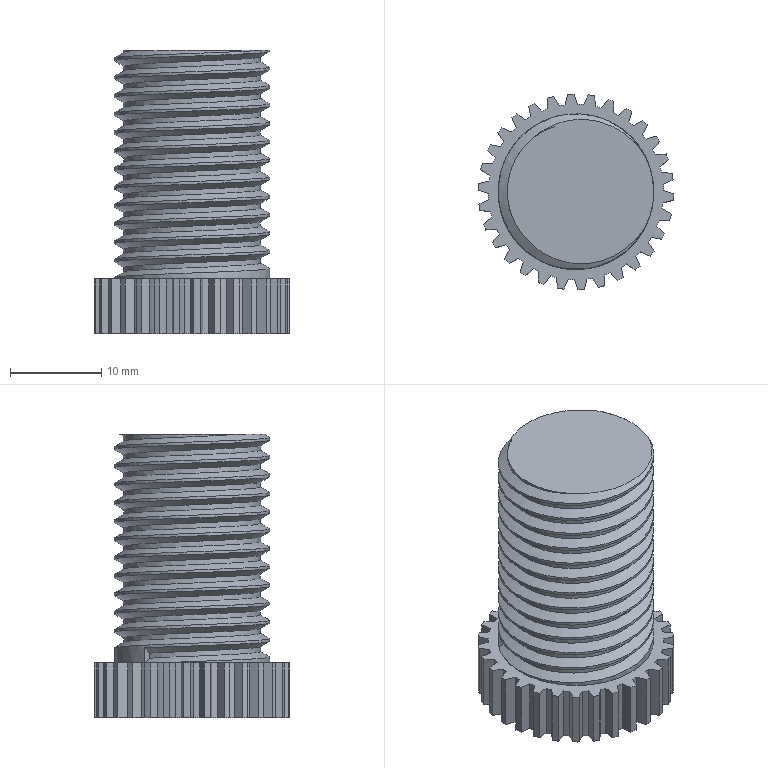Part | NX | features BREP 1, DATUM_CSYS 1, THREADS 1 | 1 solid | 129 faces | box 21.396 x 21.396 x 31 mm | volume 6909 mm3 | plane 64 | cylinder 62 | spline 3 | commonest cylinder face diameters 19.206 x30 21.4 x30 15 x1 17 x1